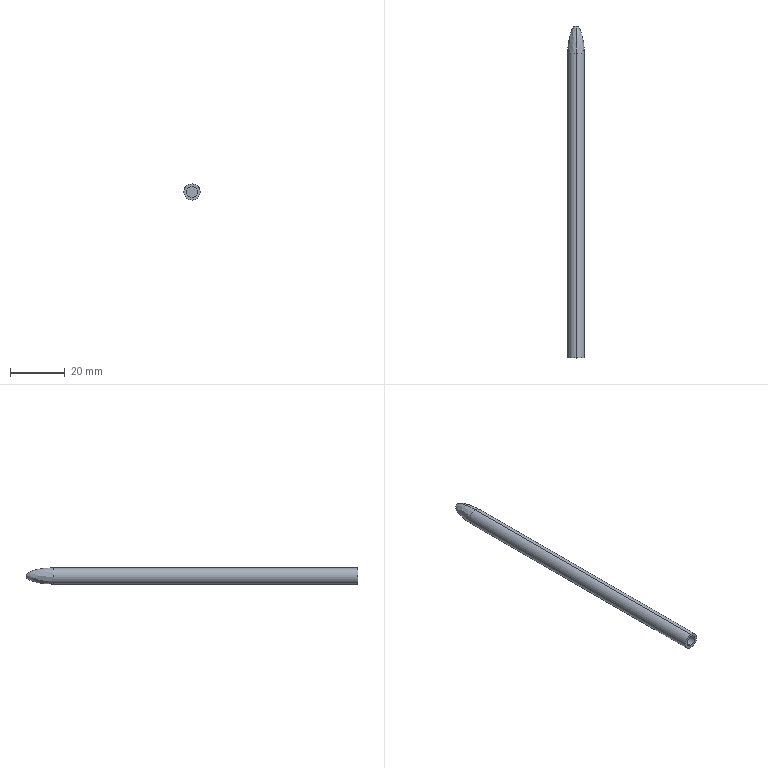Part | SolidWorks | features BaseBody 1 | 1 solid | 8 faces | box 6 x 121 x 6 mm | volume 1945 mm3 | cylinder 4 | plane 2 | spline 2 | commonest cylinder face diameters 4 x2 6 x2
STEP:
#1=CARTESIAN_POINT('',(0.,150.125,-3.));
#2=VERTEX_POINT('',#1);
#3=CARTESIAN_POINT('',(0.,150.125,3.));
#4=VERTEX_POINT('',#3);
#5=CARTESIAN_POINT('',(0.,150.125,0.));
#6=DIRECTION('',(0.,-1.,0.));
#7=DIRECTION('',(0.,0.,-1.));
#8=AXIS2_PLACEMENT_3D('',#5,#6,#7);
#9=CIRCLE('',#8,3.);
#10=EDGE_CURVE('',#2,#4,#9,.T.);
#11=ORIENTED_EDGE('',*,*,#10,.T.);
#12=CARTESIAN_POINT('',(0.,39.125,3.));
#13=VERTEX_POINT('',#12);
#14=CARTESIAN_POINT('',(0.,0.,3.));
#15=DIRECTION('',(0.,-1.,0.));
#16=VECTOR('',#15,1000.);
#17=LINE('',#14,#16);
#18=EDGE_CURVE('',#4,#13,#17,.T.);
#19=ORIENTED_EDGE('',*,*,#18,.T.);
#20=CARTESIAN_POINT('',(0.,39.125,-3.));
#21=VERTEX_POINT('',#20);
#22=CARTESIAN_POINT('',(0.,39.125,0.));
#23=DIRECTION('',(0.,1.,0.));
#24=DIRECTION('',(0.,0.,-1.));
#25=AXIS2_PLACEMENT_3D('',#22,#23,#24);
#26=CIRCLE('',#25,3.);
#27=EDGE_CURVE('',#13,#21,#26,.T.);
#28=ORIENTED_EDGE('',*,*,#27,.T.);
#29=CARTESIAN_POINT('',(0.,0.,-3.));
#30=DIRECTION('',(0.,-1.,0.));
#31=VECTOR('',#30,1000.);
#32=LINE('',#29,#31);
#33=EDGE_CURVE('',#2,#21,#32,.T.);
#34=ORIENTED_EDGE('',*,*,#33,.F.);
#35=EDGE_LOOP('',(#11,#19,#28,#34));
#36=FACE_OUTER_BOUND('',#35,.T.);
#37=CARTESIAN_POINT('',(0.,0.,0.));
#38=DIRECTION('',(0.,-1.,0.));
#39=DIRECTION('',(0.,0.,-1.));
#40=AXIS2_PLACEMENT_3D('',#37,#38,#39);
#41=CYLINDRICAL_SURFACE('',#40,3.);
#42=ADVANCED_FACE('',(#36),#41,.T.);
#43=CARTESIAN_POINT('',(0.,149.125,2.));
#44=VERTEX_POINT('',#43);
#45=CARTESIAN_POINT('',(0.,149.125,-2.));
#46=VERTEX_POINT('',#45);
#47=CARTESIAN_POINT('',(0.,149.125,0.));
#48=DIRECTION('',(0.,-1.,0.));
#49=DIRECTION('',(0.,0.,-1.));
#50=AXIS2_PLACEMENT_3D('',#47,#48,#49);
#51=CIRCLE('',#50,2.);
#52=EDGE_CURVE('',#44,#46,#51,.T.);
#53=ORIENTED_EDGE('',*,*,#52,.F.);
#54=CARTESIAN_POINT('',(0.,39.125,2.));
#55=VERTEX_POINT('',#54);
#56=CARTESIAN_POINT('',(0.,0.,2.));
#57=DIRECTION('',(0.,-1.,0.));
#58=VECTOR('',#57,1000.);
#59=LINE('',#56,#58);
#60=EDGE_CURVE('',#44,#55,#59,.T.);
#61=ORIENTED_EDGE('',*,*,#60,.T.);
#62=CARTESIAN_POINT('',(0.,39.125,-2.));
#63=VERTEX_POINT('',#62);
#64=CARTESIAN_POINT('',(0.,39.125,0.));
#65=DIRECTION('',(0.,-1.,0.));
#66=DIRECTION('',(0.,0.,-1.));
#67=AXIS2_PLACEMENT_3D('',#64,#65,#66);
#68=CIRCLE('',#67,2.);
#69=EDGE_CURVE('',#55,#63,#68,.T.);
#70=ORIENTED_EDGE('',*,*,#69,.T.);
#71=CARTESIAN_POINT('',(0.,0.,-2.));
#72=DIRECTION('',(0.,-1.,0.));
#73=VECTOR('',#72,1000.);
#74=LINE('',#71,#73);
#75=EDGE_CURVE('',#46,#63,#74,.T.);
#76=ORIENTED_EDGE('',*,*,#75,.F.);
#77=EDGE_LOOP('',(#53,#61,#70,#76));
#78=FACE_OUTER_BOUND('',#77,.T.);
#79=CARTESIAN_POINT('',(0.,0.,0.));
#80=DIRECTION('',(0.,-1.,0.));
#81=DIRECTION('',(0.,0.,-1.));
#82=AXIS2_PLACEMENT_3D('',#79,#80,#81);
#83=CYLINDRICAL_SURFACE('',#82,2.);
#84=ADVANCED_FACE('',(#78),#83,.F.);
#85=ORIENTED_EDGE('',*,*,#18,.F.);
#86=CARTESIAN_POINT('',(0.,150.125,0.));
#87=DIRECTION('',(0.,-1.,0.));
#88=DIRECTION('',(0.,0.,-1.));
#89=AXIS2_PLACEMENT_3D('',#86,#87,#88);
#90=CIRCLE('',#89,3.);
#91=EDGE_CURVE('',#4,#2,#90,.T.);
#92=ORIENTED_EDGE('',*,*,#91,.T.);
#93=ORIENTED_EDGE('',*,*,#33,.T.);
#94=CARTESIAN_POINT('',(0.,39.125,0.));
#95=DIRECTION('',(0.,1.,0.));
#96=DIRECTION('',(0.,0.,-1.));
#97=AXIS2_PLACEMENT_3D('',#94,#95,#96);
#98=CIRCLE('',#97,3.);
#99=EDGE_CURVE('',#21,#13,#98,.T.);
#100=ORIENTED_EDGE('',*,*,#99,.T.);
#101=EDGE_LOOP('',(#85,#92,#93,#100));
#102=FACE_OUTER_BOUND('',#101,.T.);
#103=CARTESIAN_POINT('',(0.,0.,0.));
#104=DIRECTION('',(0.,-1.,0.));
#105=DIRECTION('',(0.,0.,-1.));
#106=AXIS2_PLACEMENT_3D('',#103,#104,#105);
#107=CYLINDRICAL_SURFACE('',#106,3.);
#108=ADVANCED_FACE('',(#102),#107,.T.);
#109=ORIENTED_EDGE('',*,*,#99,.F.);
#110=ORIENTED_EDGE('',*,*,#27,.F.);
#111=EDGE_LOOP('',(#109,#110));
#112=FACE_OUTER_BOUND('',#111,.T.);
#113=CARTESIAN_POINT('',(0.,39.125,0.));
#114=DIRECTION('',(0.,-1.,0.));
#115=DIRECTION('',(0.,0.,-1.));
#116=AXIS2_PLACEMENT_3D('',#113,#114,#115);
#117=CIRCLE('',#116,2.);
#118=EDGE_CURVE('',#63,#55,#117,.T.);
#119=ORIENTED_EDGE('',*,*,#118,.F.);
#120=ORIENTED_EDGE('',*,*,#69,.F.);
#121=EDGE_LOOP('',(#119,#120));
#122=FACE_BOUND('',#121,.T.);
#123=CARTESIAN_POINT('',(-2.,39.125,0.));
#124=DIRECTION('',(0.,1.,0.));
#125=DIRECTION('',(0.,0.,1.));
#126=AXIS2_PLACEMENT_3D('',#123,#124,#125);
#127=PLANE('',#126);
#128=ADVANCED_FACE('',(#112,#122),#127,.F.);
#129=CARTESIAN_POINT('',(0.,160.125,0.));
#130=VERTEX_POINT('',#129);
#131=CARTESIAN_POINT('',(0.,160.125,0.));
#132=CARTESIAN_POINT('',(0.,160.125,1.757));
#133=CARTESIAN_POINT('',(0.,155.983,3.));
#134=CARTESIAN_POINT('',(0.,150.125,3.));
#135=(BOUNDED_CURVE()B_SPLINE_CURVE(3,(#131,#132,#133,#134),.UNSPECIFIED.,.F.,.T.)B_SPLINE_CURVE_WITH_KNOTS((4,4),(0.,1.),.UNSPECIFIED.)CURVE()GEOMETRIC_REPRESENTATION_ITEM()RATIONAL_B_SPLINE_CURVE((1.,0.8047,0.8047,1.))REPRESENTATION_ITEM(''));
#136=EDGE_CURVE('',#130,#4,#135,.T.);
#137=ORIENTED_EDGE('',*,*,#136,.T.);
#138=ORIENTED_EDGE('',*,*,#10,.F.);
#139=CARTESIAN_POINT('',(0.,150.125,-3.));
#140=CARTESIAN_POINT('',(0.,155.983,-3.));
#141=CARTESIAN_POINT('',(0.,160.125,-1.757));
#142=CARTESIAN_POINT('',(0.,160.125,0.));
#143=(BOUNDED_CURVE()B_SPLINE_CURVE(3,(#139,#140,#141,#142),.UNSPECIFIED.,.F.,.F.)B_SPLINE_CURVE_WITH_KNOTS((4,4),(0.,1.),.UNSPECIFIED.)CURVE()GEOMETRIC_REPRESENTATION_ITEM()RATIONAL_B_SPLINE_CURVE((1.,0.8047,0.8047,1.))REPRESENTATION_ITEM(''));
#144=EDGE_CURVE('',#2,#130,#143,.T.);
#145=ORIENTED_EDGE('',*,*,#144,.T.);
#146=EDGE_LOOP('',(#137,#138,#145));
#147=FACE_OUTER_BOUND('',#146,.T.);
#148=CARTESIAN_POINT('',(0.,160.125,0.));
#149=CARTESIAN_POINT('',(0.,160.125,0.));
#150=CARTESIAN_POINT('',(0.,160.125,0.));
#151=CARTESIAN_POINT('',(0.,160.125,0.));
#152=CARTESIAN_POINT('',(0.,160.125,1.757));
#153=CARTESIAN_POINT('',(3.515,160.125,1.757));
#154=CARTESIAN_POINT('',(3.515,160.125,-1.757));
#155=CARTESIAN_POINT('',(0.,160.125,-1.757));
#156=CARTESIAN_POINT('',(0.,155.983,3.));
#157=CARTESIAN_POINT('',(6.,155.983,3.));
#158=CARTESIAN_POINT('',(6.,155.983,-3.));
#159=CARTESIAN_POINT('',(0.,155.983,-3.));
#160=CARTESIAN_POINT('',(0.,150.125,3.));
#161=CARTESIAN_POINT('',(6.,150.125,3.));
#162=CARTESIAN_POINT('',(6.,150.125,-3.));
#163=CARTESIAN_POINT('',(0.,150.125,-3.));
#164=(BOUNDED_SURFACE()B_SPLINE_SURFACE(3,3,((#148,#149,#150,#151),(#152,#153,#154,#155),(#156,#157,#158,#159),(#160,#161,#162,#163)),.UNSPECIFIED.,.F.,.F.,.F.)B_SPLINE_SURFACE_WITH_KNOTS((4,4),(4,4),(0.,1.),(0.,1.),.UNSPECIFIED.)GEOMETRIC_REPRESENTATION_ITEM()RATIONAL_B_SPLINE_SURFACE(((1.,0.3333,0.3333,1.),(0.8047,0.2682,0.2682,0.8047),(0.8047,0.2682,0.2682,0.8047),(1.,0.3333,0.3333,1.)))REPRESENTATION_ITEM('')SURFACE());
#165=ADVANCED_FACE('',(#147),#164,.T.);
#166=ORIENTED_EDGE('',*,*,#144,.F.);
#167=ORIENTED_EDGE('',*,*,#91,.F.);
#168=ORIENTED_EDGE('',*,*,#136,.F.);
#169=EDGE_LOOP('',(#166,#167,#168));
#170=FACE_OUTER_BOUND('',#169,.T.);
#171=CARTESIAN_POINT('',(0.,160.125,0.));
#172=CARTESIAN_POINT('',(0.,160.125,0.));
#173=CARTESIAN_POINT('',(0.,160.125,0.));
#174=CARTESIAN_POINT('',(0.,160.125,0.));
#175=CARTESIAN_POINT('',(0.,160.125,-1.757));
#176=CARTESIAN_POINT('',(-3.515,160.125,-1.757));
#177=CARTESIAN_POINT('',(-3.515,160.125,1.757));
#178=CARTESIAN_POINT('',(0.,160.125,1.757));
#179=CARTESIAN_POINT('',(0.,155.983,-3.));
#180=CARTESIAN_POINT('',(-6.,155.983,-3.));
#181=CARTESIAN_POINT('',(-6.,155.983,3.));
#182=CARTESIAN_POINT('',(0.,155.983,3.));
#183=CARTESIAN_POINT('',(0.,150.125,-3.));
#184=CARTESIAN_POINT('',(-6.,150.125,-3.));
#185=CARTESIAN_POINT('',(-6.,150.125,3.));
#186=CARTESIAN_POINT('',(0.,150.125,3.));
#187=(BOUNDED_SURFACE()B_SPLINE_SURFACE(3,3,((#171,#172,#173,#174),(#175,#176,#177,#178),(#179,#180,#181,#182),(#183,#184,#185,#186)),.UNSPECIFIED.,.F.,.F.,.F.)B_SPLINE_SURFACE_WITH_KNOTS((4,4),(4,4),(0.,1.),(0.,1.),.UNSPECIFIED.)GEOMETRIC_REPRESENTATION_ITEM()RATIONAL_B_SPLINE_SURFACE(((1.,0.3333,0.3333,1.),(0.8047,0.2682,0.2682,0.8047),(0.8047,0.2682,0.2682,0.8047),(1.,0.3333,0.3333,1.)))REPRESENTATION_ITEM('')SURFACE());
#188=ADVANCED_FACE('',(#170),#187,.T.);
#189=ORIENTED_EDGE('',*,*,#60,.F.);
#190=CARTESIAN_POINT('',(0.,149.125,0.));
#191=DIRECTION('',(0.,-1.,0.));
#192=DIRECTION('',(0.,0.,-1.));
#193=AXIS2_PLACEMENT_3D('',#190,#191,#192);
#194=CIRCLE('',#193,2.);
#195=EDGE_CURVE('',#46,#44,#194,.T.);
#196=ORIENTED_EDGE('',*,*,#195,.F.);
#197=ORIENTED_EDGE('',*,*,#75,.T.);
#198=ORIENTED_EDGE('',*,*,#118,.T.);
#199=EDGE_LOOP('',(#189,#196,#197,#198));
#200=FACE_OUTER_BOUND('',#199,.T.);
#201=CARTESIAN_POINT('',(0.,0.,0.));
#202=DIRECTION('',(0.,-1.,0.));
#203=DIRECTION('',(0.,0.,-1.));
#204=AXIS2_PLACEMENT_3D('',#201,#202,#203);
#205=CYLINDRICAL_SURFACE('',#204,2.);
#206=ADVANCED_FACE('',(#200),#205,.F.);
#207=ORIENTED_EDGE('',*,*,#195,.T.);
#208=ORIENTED_EDGE('',*,*,#52,.T.);
#209=EDGE_LOOP('',(#207,#208));
#210=FACE_OUTER_BOUND('',#209,.T.);
#211=CARTESIAN_POINT('',(0.,149.125,0.));
#212=DIRECTION('',(0.,1.,0.));
#213=DIRECTION('',(0.,0.,1.));
#214=AXIS2_PLACEMENT_3D('',#211,#212,#213);
#215=PLANE('',#214);
#216=ADVANCED_FACE('',(#210),#215,.F.);
#217=CLOSED_SHELL('',(#42,#84,#108,#128,#165,#188,#206,#216));
#218=MANIFOLD_SOLID_BREP('',#217);
#219=CARTESIAN_POINT('',(0.,0.,0.));
#220=DIRECTION('',(0.,0.,1.));
#221=DIRECTION('',(1.,0.,0.));
#222=AXIS2_PLACEMENT_3D('',#219,#220,#221);
#223=(LENGTH_UNIT()NAMED_UNIT(*)SI_UNIT(.MILLI.,.METRE.));
#224=UNCERTAINTY_MEASURE_WITH_UNIT(LENGTH_MEASURE(0.00001),#223,'','');
#225=(NAMED_UNIT(*)PLANE_ANGLE_UNIT()SI_UNIT($,.RADIAN.));
#226=(NAMED_UNIT(*)SI_UNIT($,.STERADIAN.)SOLID_ANGLE_UNIT());
#227=(GEOMETRIC_REPRESENTATION_CONTEXT(3)GLOBAL_UNCERTAINTY_ASSIGNED_CONTEXT((#224))GLOBAL_UNIT_ASSIGNED_CONTEXT((#223,#225,#226))REPRESENTATION_CONTEXT('',''));
#228=ADVANCED_BREP_SHAPE_REPRESENTATION('',(#218,#222),#227);